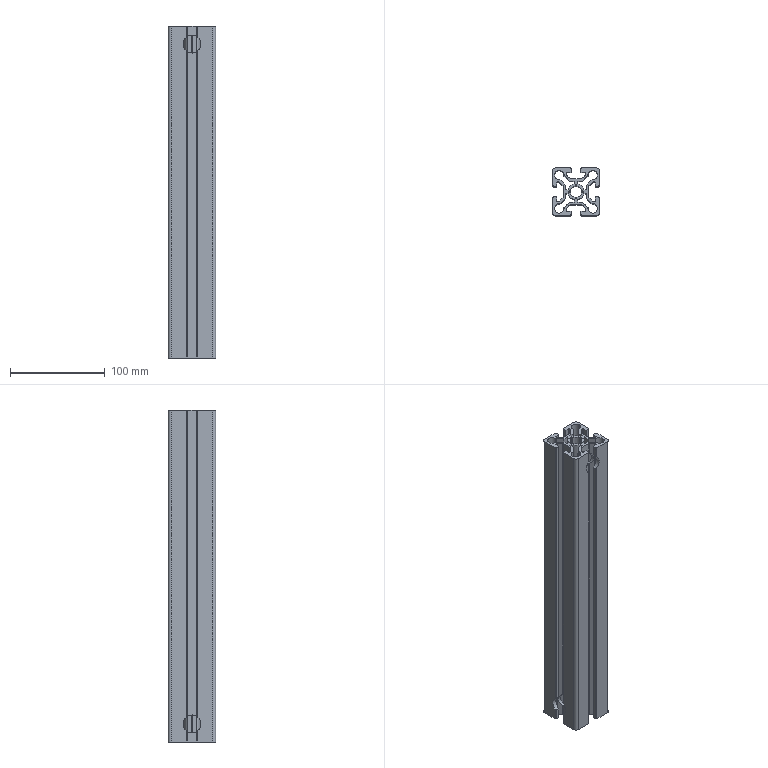Part | NX | features BREP 1 | 1 solid | 231 faces | box 50 x 50 x 350 mm | volume 340655 mm3 | plane 154 | cylinder 77 | commonest cylinder face diameters 2 x37 19 x16 10 x12 6 x4 12 x4 17 x4